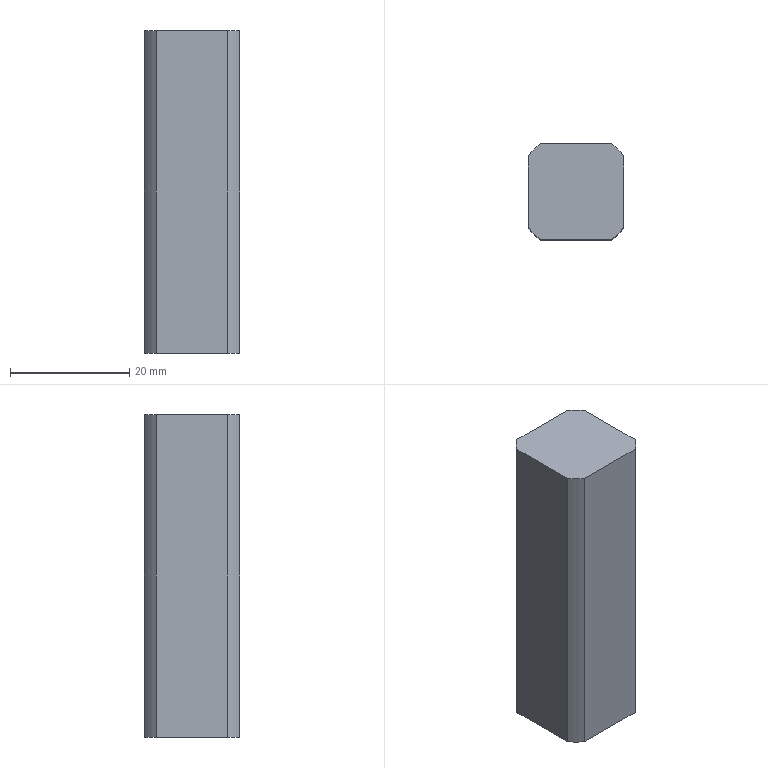Part | STEP file | _CKZT40_ARM.stp | 1 solid | 10 faces | box 16 x 16 x 54 mm | volume 13433 mm3 | plane 6 | cylinder 4 | commonest cylinder face diameters 20 x4
STEP:
#1=CARTESIAN_POINT('',(0.,0.,0.));
#2=DIRECTION('',(0.,0.,1.));
#3=DIRECTION('',(1.,0.,0.));
#4=AXIS2_PLACEMENT_3D('',#1,#2,#3);
#5=CARTESIAN_POINT('',(-6.,8.,27.));
#6=VERTEX_POINT('',#5);
#7=CARTESIAN_POINT('',(-8.,6.,27.));
#8=VERTEX_POINT('',#7);
#9=CARTESIAN_POINT('',(0.,0.,27.));
#10=DIRECTION('',(0.,0.,1.));
#11=DIRECTION('',(1.,0.,0.));
#12=AXIS2_PLACEMENT_3D('',#9,#10,#11);
#13=CIRCLE('',#12,10.);
#14=CARTESIAN_POINT('',(-8.8,-8.8,27.));
#15=DIRECTION('',(0.,0.,1.));
#16=DIRECTION('',(1.,0.,0.));
#17=AXIS2_PLACEMENT_3D('',#14,#15,#16);
#18=PLANE('',#17);
#19=CARTESIAN_POINT('',(8.8,8.8));
#20=DIRECTION('',(1.,0.));
#21=AXIS2_PLACEMENT_2D('',#19,#20);
#22=CIRCLE('',#21,10.);
#23=(GEOMETRIC_REPRESENTATION_CONTEXT(2)PARAMETRIC_REPRESENTATION_CONTEXT()REPRESENTATION_CONTEXT('',''));
#24=DEFINITIONAL_REPRESENTATION('',(#22),#23);
#25=PCURVE('',#18,#24);
#26=CARTESIAN_POINT('',(0.,0.,-29.7));
#27=DIRECTION('',(0.,0.,1.));
#28=DIRECTION('',(-1.,0.,0.));
#29=AXIS2_PLACEMENT_3D('',#26,#27,#28);
#30=CYLINDRICAL_SURFACE('',#29,10.);
#31=CARTESIAN_POINT('',(3.142,56.7));
#32=DIRECTION('',(1.,0.));
#33=VECTOR('',#32,1.);
#34=LINE('',#31,#33);
#35=(GEOMETRIC_REPRESENTATION_CONTEXT(2)PARAMETRIC_REPRESENTATION_CONTEXT()REPRESENTATION_CONTEXT('',''));
#36=DEFINITIONAL_REPRESENTATION('',(#34),#35);
#37=PCURVE('',#30,#36);
#38=SURFACE_CURVE('',#13,(#25,#37),.PCURVE_S1.);
#39=EDGE_CURVE('',#6,#8,#38,.T.);
#40=ORIENTED_EDGE('',*,*,#39,.T.);
#41=CARTESIAN_POINT('',(-8.,-6.,27.));
#42=VERTEX_POINT('',#41);
#43=CARTESIAN_POINT('',(-8.,6.,27.));
#44=DIRECTION('',(0.,-1.,0.));
#45=VECTOR('',#44,1.);
#46=LINE('',#43,#45);
#47=CARTESIAN_POINT('',(0.8,14.8));
#48=DIRECTION('',(0.,-1.));
#49=VECTOR('',#48,1.);
#50=LINE('',#47,#49);
#51=(GEOMETRIC_REPRESENTATION_CONTEXT(2)PARAMETRIC_REPRESENTATION_CONTEXT()REPRESENTATION_CONTEXT('',''));
#52=DEFINITIONAL_REPRESENTATION('',(#50),#51);
#53=PCURVE('',#18,#52);
#54=CARTESIAN_POINT('',(-8.,-6.6,29.7));
#55=DIRECTION('',(1.,0.,0.));
#56=DIRECTION('',(0.,1.,0.));
#57=AXIS2_PLACEMENT_3D('',#54,#55,#56);
#58=PLANE('',#57);
#59=CARTESIAN_POINT('',(12.6,-2.7));
#60=DIRECTION('',(-1.,0.));
#61=VECTOR('',#60,1.);
#62=LINE('',#59,#61);
#63=(GEOMETRIC_REPRESENTATION_CONTEXT(2)PARAMETRIC_REPRESENTATION_CONTEXT()REPRESENTATION_CONTEXT('',''));
#64=DEFINITIONAL_REPRESENTATION('',(#62),#63);
#65=PCURVE('',#58,#64);
#66=SURFACE_CURVE('',#46,(#53,#65),.PCURVE_S1.);
#67=EDGE_CURVE('',#8,#42,#66,.T.);
#68=ORIENTED_EDGE('',*,*,#67,.T.);
#69=CARTESIAN_POINT('',(-6.,-8.,27.));
#70=VERTEX_POINT('',#69);
#71=CARTESIAN_POINT('',(0.,0.,27.));
#72=DIRECTION('',(0.,0.,1.));
#73=DIRECTION('',(1.,0.,0.));
#74=AXIS2_PLACEMENT_3D('',#71,#72,#73);
#75=CIRCLE('',#74,10.);
#76=CARTESIAN_POINT('',(8.8,8.8));
#77=DIRECTION('',(1.,0.));
#78=AXIS2_PLACEMENT_2D('',#76,#77);
#79=CIRCLE('',#78,10.);
#80=(GEOMETRIC_REPRESENTATION_CONTEXT(2)PARAMETRIC_REPRESENTATION_CONTEXT()REPRESENTATION_CONTEXT('',''));
#81=DEFINITIONAL_REPRESENTATION('',(#79),#80);
#82=PCURVE('',#18,#81);
#83=CARTESIAN_POINT('',(0.,0.,-29.7));
#84=DIRECTION('',(0.,0.,1.));
#85=DIRECTION('',(-1.,0.,0.));
#86=AXIS2_PLACEMENT_3D('',#83,#84,#85);
#87=CYLINDRICAL_SURFACE('',#86,10.);
#88=CARTESIAN_POINT('',(-3.142,56.7));
#89=DIRECTION('',(1.,0.));
#90=VECTOR('',#89,1.);
#91=LINE('',#88,#90);
#92=(GEOMETRIC_REPRESENTATION_CONTEXT(2)PARAMETRIC_REPRESENTATION_CONTEXT()REPRESENTATION_CONTEXT('',''));
#93=DEFINITIONAL_REPRESENTATION('',(#91),#92);
#94=PCURVE('',#87,#93);
#95=SURFACE_CURVE('',#75,(#82,#94),.PCURVE_S1.);
#96=EDGE_CURVE('',#42,#70,#95,.T.);
#97=ORIENTED_EDGE('',*,*,#96,.T.);
#98=CARTESIAN_POINT('',(6.,-8.,27.));
#99=VERTEX_POINT('',#98);
#100=CARTESIAN_POINT('',(-6.,-8.,27.));
#101=DIRECTION('',(1.,0.,0.));
#102=VECTOR('',#101,1.);
#103=LINE('',#100,#102);
#104=CARTESIAN_POINT('',(2.8,0.8));
#105=DIRECTION('',(1.,0.));
#106=VECTOR('',#105,1.);
#107=LINE('',#104,#106);
#108=(GEOMETRIC_REPRESENTATION_CONTEXT(2)PARAMETRIC_REPRESENTATION_CONTEXT()REPRESENTATION_CONTEXT('',''));
#109=DEFINITIONAL_REPRESENTATION('',(#107),#108);
#110=PCURVE('',#18,#109);
#111=CARTESIAN_POINT('',(-6.6,-8.,-29.7));
#112=DIRECTION('',(0.,1.,0.));
#113=DIRECTION('',(1.,0.,0.));
#114=AXIS2_PLACEMENT_3D('',#111,#112,#113);
#115=PLANE('',#114);
#116=CARTESIAN_POINT('',(0.6,-56.7));
#117=DIRECTION('',(1.,0.));
#118=VECTOR('',#117,1.);
#119=LINE('',#116,#118);
#120=(GEOMETRIC_REPRESENTATION_CONTEXT(2)PARAMETRIC_REPRESENTATION_CONTEXT()REPRESENTATION_CONTEXT('',''));
#121=DEFINITIONAL_REPRESENTATION('',(#119),#120);
#122=PCURVE('',#115,#121);
#123=SURFACE_CURVE('',#103,(#110,#122),.PCURVE_S1.);
#124=EDGE_CURVE('',#70,#99,#123,.T.);
#125=ORIENTED_EDGE('',*,*,#124,.T.);
#126=CARTESIAN_POINT('',(8.,-6.,27.));
#127=VERTEX_POINT('',#126);
#128=CARTESIAN_POINT('',(0.,0.,27.));
#129=DIRECTION('',(0.,0.,1.));
#130=DIRECTION('',(1.,0.,0.));
#131=AXIS2_PLACEMENT_3D('',#128,#129,#130);
#132=CIRCLE('',#131,10.);
#133=CARTESIAN_POINT('',(8.8,8.8));
#134=DIRECTION('',(1.,0.));
#135=AXIS2_PLACEMENT_2D('',#133,#134);
#136=CIRCLE('',#135,10.);
#137=(GEOMETRIC_REPRESENTATION_CONTEXT(2)PARAMETRIC_REPRESENTATION_CONTEXT()REPRESENTATION_CONTEXT('',''));
#138=DEFINITIONAL_REPRESENTATION('',(#136),#137);
#139=PCURVE('',#18,#138);
#140=CARTESIAN_POINT('',(0.,0.,-29.7));
#141=DIRECTION('',(0.,0.,1.));
#142=DIRECTION('',(-1.,0.,0.));
#143=AXIS2_PLACEMENT_3D('',#140,#141,#142);
#144=CYLINDRICAL_SURFACE('',#143,10.);
#145=CARTESIAN_POINT('',(-3.142,56.7));
#146=DIRECTION('',(1.,0.));
#147=VECTOR('',#146,1.);
#148=LINE('',#145,#147);
#149=(GEOMETRIC_REPRESENTATION_CONTEXT(2)PARAMETRIC_REPRESENTATION_CONTEXT()REPRESENTATION_CONTEXT('',''));
#150=DEFINITIONAL_REPRESENTATION('',(#148),#149);
#151=PCURVE('',#144,#150);
#152=SURFACE_CURVE('',#132,(#139,#151),.PCURVE_S1.);
#153=EDGE_CURVE('',#99,#127,#152,.T.);
#154=ORIENTED_EDGE('',*,*,#153,.T.);
#155=CARTESIAN_POINT('',(8.,6.,27.));
#156=VERTEX_POINT('',#155);
#157=CARTESIAN_POINT('',(8.,-6.,27.));
#158=DIRECTION('',(0.,1.,0.));
#159=VECTOR('',#158,1.);
#160=LINE('',#157,#159);
#161=CARTESIAN_POINT('',(16.8,2.8));
#162=DIRECTION('',(0.,1.));
#163=VECTOR('',#162,1.);
#164=LINE('',#161,#163);
#165=(GEOMETRIC_REPRESENTATION_CONTEXT(2)PARAMETRIC_REPRESENTATION_CONTEXT()REPRESENTATION_CONTEXT('',''));
#166=DEFINITIONAL_REPRESENTATION('',(#164),#165);
#167=PCURVE('',#18,#166);
#168=CARTESIAN_POINT('',(8.,-6.6,-29.7));
#169=DIRECTION('',(-1.,0.,0.));
#170=DIRECTION('',(0.,0.,1.));
#171=AXIS2_PLACEMENT_3D('',#168,#169,#170);
#172=PLANE('',#171);
#173=CARTESIAN_POINT('',(56.7,0.6));
#174=DIRECTION('',(0.,1.));
#175=VECTOR('',#174,1.);
#176=LINE('',#173,#175);
#177=(GEOMETRIC_REPRESENTATION_CONTEXT(2)PARAMETRIC_REPRESENTATION_CONTEXT()REPRESENTATION_CONTEXT('',''));
#178=DEFINITIONAL_REPRESENTATION('',(#176),#177);
#179=PCURVE('',#172,#178);
#180=SURFACE_CURVE('',#160,(#167,#179),.PCURVE_S1.);
#181=EDGE_CURVE('',#127,#156,#180,.T.);
#182=ORIENTED_EDGE('',*,*,#181,.T.);
#183=CARTESIAN_POINT('',(6.,8.,27.));
#184=VERTEX_POINT('',#183);
#185=CARTESIAN_POINT('',(0.,0.,27.));
#186=DIRECTION('',(0.,0.,1.));
#187=DIRECTION('',(1.,0.,0.));
#188=AXIS2_PLACEMENT_3D('',#185,#186,#187);
#189=CIRCLE('',#188,10.);
#190=CARTESIAN_POINT('',(8.8,8.8));
#191=DIRECTION('',(1.,0.));
#192=AXIS2_PLACEMENT_2D('',#190,#191);
#193=CIRCLE('',#192,10.);
#194=(GEOMETRIC_REPRESENTATION_CONTEXT(2)PARAMETRIC_REPRESENTATION_CONTEXT()REPRESENTATION_CONTEXT('',''));
#195=DEFINITIONAL_REPRESENTATION('',(#193),#194);
#196=PCURVE('',#18,#195);
#197=CARTESIAN_POINT('',(0.,0.,-29.7));
#198=DIRECTION('',(0.,0.,1.));
#199=DIRECTION('',(-1.,0.,0.));
#200=AXIS2_PLACEMENT_3D('',#197,#198,#199);
#201=CYLINDRICAL_SURFACE('',#200,10.);
#202=CARTESIAN_POINT('',(3.142,56.7));
#203=DIRECTION('',(1.,0.));
#204=VECTOR('',#203,1.);
#205=LINE('',#202,#204);
#206=(GEOMETRIC_REPRESENTATION_CONTEXT(2)PARAMETRIC_REPRESENTATION_CONTEXT()REPRESENTATION_CONTEXT('',''));
#207=DEFINITIONAL_REPRESENTATION('',(#205),#206);
#208=PCURVE('',#201,#207);
#209=SURFACE_CURVE('',#189,(#196,#208),.PCURVE_S1.);
#210=EDGE_CURVE('',#156,#184,#209,.T.);
#211=ORIENTED_EDGE('',*,*,#210,.T.);
#212=CARTESIAN_POINT('',(6.,8.,27.));
#213=DIRECTION('',(-1.,0.,0.));
#214=VECTOR('',#213,1.);
#215=LINE('',#212,#214);
#216=CARTESIAN_POINT('',(14.8,16.8));
#217=DIRECTION('',(-1.,0.));
#218=VECTOR('',#217,1.);
#219=LINE('',#216,#218);
#220=(GEOMETRIC_REPRESENTATION_CONTEXT(2)PARAMETRIC_REPRESENTATION_CONTEXT()REPRESENTATION_CONTEXT('',''));
#221=DEFINITIONAL_REPRESENTATION('',(#219),#220);
#222=PCURVE('',#18,#221);
#223=CARTESIAN_POINT('',(-6.6,8.,29.7));
#224=DIRECTION('',(0.,-1.,0.));
#225=DIRECTION('',(0.,0.,-1.));
#226=AXIS2_PLACEMENT_3D('',#223,#224,#225);
#227=PLANE('',#226);
#228=CARTESIAN_POINT('',(2.7,12.6));
#229=DIRECTION('',(0.,-1.));
#230=VECTOR('',#229,1.);
#231=LINE('',#228,#230);
#232=(GEOMETRIC_REPRESENTATION_CONTEXT(2)PARAMETRIC_REPRESENTATION_CONTEXT()REPRESENTATION_CONTEXT('',''));
#233=DEFINITIONAL_REPRESENTATION('',(#231),#232);
#234=PCURVE('',#227,#233);
#235=SURFACE_CURVE('',#215,(#222,#234),.PCURVE_S1.);
#236=EDGE_CURVE('',#184,#6,#235,.T.);
#237=ORIENTED_EDGE('',*,*,#236,.T.);
#238=EDGE_LOOP('',(#40,#68,#97,#125,#154,#182,#211,#237));
#239=FACE_BOUND('',#238,.T.);
#240=ADVANCED_FACE('',(#239),#18,.T.);
#241=CARTESIAN_POINT('',(-6.,8.,-27.));
#242=VERTEX_POINT('',#241);
#243=CARTESIAN_POINT('',(-8.,6.,-27.));
#244=VERTEX_POINT('',#243);
#245=CARTESIAN_POINT('',(0.,0.,-27.));
#246=DIRECTION('',(0.,0.,1.));
#247=DIRECTION('',(1.,0.,0.));
#248=AXIS2_PLACEMENT_3D('',#245,#246,#247);
#249=CIRCLE('',#248,10.);
#250=CARTESIAN_POINT('',(-8.8,-8.8,-27.));
#251=DIRECTION('',(0.,0.,1.));
#252=DIRECTION('',(1.,0.,0.));
#253=AXIS2_PLACEMENT_3D('',#250,#251,#252);
#254=PLANE('',#253);
#255=CARTESIAN_POINT('',(8.8,8.8));
#256=DIRECTION('',(1.,0.));
#257=AXIS2_PLACEMENT_2D('',#255,#256);
#258=CIRCLE('',#257,10.);
#259=(GEOMETRIC_REPRESENTATION_CONTEXT(2)PARAMETRIC_REPRESENTATION_CONTEXT()REPRESENTATION_CONTEXT('',''));
#260=DEFINITIONAL_REPRESENTATION('',(#258),#259);
#261=PCURVE('',#254,#260);
#262=CARTESIAN_POINT('',(3.142,2.7));
#263=DIRECTION('',(1.,0.));
#264=VECTOR('',#263,1.);
#265=LINE('',#262,#264);
#266=(GEOMETRIC_REPRESENTATION_CONTEXT(2)PARAMETRIC_REPRESENTATION_CONTEXT()REPRESENTATION_CONTEXT('',''));
#267=DEFINITIONAL_REPRESENTATION('',(#265),#266);
#268=PCURVE('',#30,#267);
#269=SURFACE_CURVE('',#249,(#261,#268),.PCURVE_S1.);
#270=EDGE_CURVE('',#242,#244,#269,.T.);
#271=ORIENTED_EDGE('',*,*,#270,.F.);
#272=CARTESIAN_POINT('',(6.,8.,-27.));
#273=VERTEX_POINT('',#272);
#274=CARTESIAN_POINT('',(6.,8.,-27.));
#275=DIRECTION('',(-1.,0.,0.));
#276=VECTOR('',#275,1.);
#277=LINE('',#274,#276);
#278=CARTESIAN_POINT('',(14.8,16.8));
#279=DIRECTION('',(-1.,0.));
#280=VECTOR('',#279,1.);
#281=LINE('',#278,#280);
#282=(GEOMETRIC_REPRESENTATION_CONTEXT(2)PARAMETRIC_REPRESENTATION_CONTEXT()REPRESENTATION_CONTEXT('',''));
#283=DEFINITIONAL_REPRESENTATION('',(#281),#282);
#284=PCURVE('',#254,#283);
#285=CARTESIAN_POINT('',(56.7,12.6));
#286=DIRECTION('',(0.,-1.));
#287=VECTOR('',#286,1.);
#288=LINE('',#285,#287);
#289=(GEOMETRIC_REPRESENTATION_CONTEXT(2)PARAMETRIC_REPRESENTATION_CONTEXT()REPRESENTATION_CONTEXT('',''));
#290=DEFINITIONAL_REPRESENTATION('',(#288),#289);
#291=PCURVE('',#227,#290);
#292=SURFACE_CURVE('',#277,(#284,#291),.PCURVE_S1.);
#293=EDGE_CURVE('',#273,#242,#292,.T.);
#294=ORIENTED_EDGE('',*,*,#293,.F.);
#295=CARTESIAN_POINT('',(8.,6.,-27.));
#296=VERTEX_POINT('',#295);
#297=CARTESIAN_POINT('',(0.,0.,-27.));
#298=DIRECTION('',(0.,0.,1.));
#299=DIRECTION('',(1.,0.,0.));
#300=AXIS2_PLACEMENT_3D('',#297,#298,#299);
#301=CIRCLE('',#300,10.);
#302=CARTESIAN_POINT('',(8.8,8.8));
#303=DIRECTION('',(1.,0.));
#304=AXIS2_PLACEMENT_2D('',#302,#303);
#305=CIRCLE('',#304,10.);
#306=(GEOMETRIC_REPRESENTATION_CONTEXT(2)PARAMETRIC_REPRESENTATION_CONTEXT()REPRESENTATION_CONTEXT('',''));
#307=DEFINITIONAL_REPRESENTATION('',(#305),#306);
#308=PCURVE('',#254,#307);
#309=CARTESIAN_POINT('',(3.142,2.7));
#310=DIRECTION('',(1.,0.));
#311=VECTOR('',#310,1.);
#312=LINE('',#309,#311);
#313=(GEOMETRIC_REPRESENTATION_CONTEXT(2)PARAMETRIC_REPRESENTATION_CONTEXT()REPRESENTATION_CONTEXT('',''));
#314=DEFINITIONAL_REPRESENTATION('',(#312),#313);
#315=PCURVE('',#201,#314);
#316=SURFACE_CURVE('',#301,(#308,#315),.PCURVE_S1.);
#317=EDGE_CURVE('',#296,#273,#316,.T.);
#318=ORIENTED_EDGE('',*,*,#317,.F.);
#319=CARTESIAN_POINT('',(8.,-6.,-27.));
#320=VERTEX_POINT('',#319);
#321=CARTESIAN_POINT('',(8.,-6.,-27.));
#322=DIRECTION('',(0.,1.,0.));
#323=VECTOR('',#322,1.);
#324=LINE('',#321,#323);
#325=CARTESIAN_POINT('',(16.8,2.8));
#326=DIRECTION('',(0.,1.));
#327=VECTOR('',#326,1.);
#328=LINE('',#325,#327);
#329=(GEOMETRIC_REPRESENTATION_CONTEXT(2)PARAMETRIC_REPRESENTATION_CONTEXT()REPRESENTATION_CONTEXT('',''));
#330=DEFINITIONAL_REPRESENTATION('',(#328),#329);
#331=PCURVE('',#254,#330);
#332=CARTESIAN_POINT('',(2.7,0.6));
#333=DIRECTION('',(0.,1.));
#334=VECTOR('',#333,1.);
#335=LINE('',#332,#334);
#336=(GEOMETRIC_REPRESENTATION_CONTEXT(2)PARAMETRIC_REPRESENTATION_CONTEXT()REPRESENTATION_CONTEXT('',''));
#337=DEFINITIONAL_REPRESENTATION('',(#335),#336);
#338=PCURVE('',#172,#337);
#339=SURFACE_CURVE('',#324,(#331,#338),.PCURVE_S1.);
#340=EDGE_CURVE('',#320,#296,#339,.T.);
#341=ORIENTED_EDGE('',*,*,#340,.F.);
#342=CARTESIAN_POINT('',(6.,-8.,-27.));
#343=VERTEX_POINT('',#342);
#344=CARTESIAN_POINT('',(0.,0.,-27.));
#345=DIRECTION('',(0.,0.,1.));
#346=DIRECTION('',(1.,0.,0.));
#347=AXIS2_PLACEMENT_3D('',#344,#345,#346);
#348=CIRCLE('',#347,10.);
#349=CARTESIAN_POINT('',(8.8,8.8));
#350=DIRECTION('',(1.,0.));
#351=AXIS2_PLACEMENT_2D('',#349,#350);
#352=CIRCLE('',#351,10.);
#353=(GEOMETRIC_REPRESENTATION_CONTEXT(2)PARAMETRIC_REPRESENTATION_CONTEXT()REPRESENTATION_CONTEXT('',''));
#354=DEFINITIONAL_REPRESENTATION('',(#352),#353);
#355=PCURVE('',#254,#354);
#356=CARTESIAN_POINT('',(-3.142,2.7));
#357=DIRECTION('',(1.,0.));
#358=VECTOR('',#357,1.);
#359=LINE('',#356,#358);
#360=(GEOMETRIC_REPRESENTATION_CONTEXT(2)PARAMETRIC_REPRESENTATION_CONTEXT()REPRESENTATION_CONTEXT('',''));
#361=DEFINITIONAL_REPRESENTATION('',(#359),#360);
#362=PCURVE('',#144,#361);
#363=SURFACE_CURVE('',#348,(#355,#362),.PCURVE_S1.);
#364=EDGE_CURVE('',#343,#320,#363,.T.);
#365=ORIENTED_EDGE('',*,*,#364,.F.);
#366=CARTESIAN_POINT('',(-6.,-8.,-27.));
#367=VERTEX_POINT('',#366);
#368=CARTESIAN_POINT('',(-6.,-8.,-27.));
#369=DIRECTION('',(1.,0.,0.));
#370=VECTOR('',#369,1.);
#371=LINE('',#368,#370);
#372=CARTESIAN_POINT('',(2.8,0.8));
#373=DIRECTION('',(1.,0.));
#374=VECTOR('',#373,1.);
#375=LINE('',#372,#374);
#376=(GEOMETRIC_REPRESENTATION_CONTEXT(2)PARAMETRIC_REPRESENTATION_CONTEXT()REPRESENTATION_CONTEXT('',''));
#377=DEFINITIONAL_REPRESENTATION('',(#375),#376);
#378=PCURVE('',#254,#377);
#379=CARTESIAN_POINT('',(0.6,-2.7));
#380=DIRECTION('',(1.,0.));
#381=VECTOR('',#380,1.);
#382=LINE('',#379,#381);
#383=(GEOMETRIC_REPRESENTATION_CONTEXT(2)PARAMETRIC_REPRESENTATION_CONTEXT()REPRESENTATION_CONTEXT('',''));
#384=DEFINITIONAL_REPRESENTATION('',(#382),#383);
#385=PCURVE('',#115,#384);
#386=SURFACE_CURVE('',#371,(#378,#385),.PCURVE_S1.);
#387=EDGE_CURVE('',#367,#343,#386,.T.);
#388=ORIENTED_EDGE('',*,*,#387,.F.);
#389=CARTESIAN_POINT('',(-8.,-6.,-27.));
#390=VERTEX_POINT('',#389);
#391=CARTESIAN_POINT('',(0.,0.,-27.));
#392=DIRECTION('',(0.,0.,1.));
#393=DIRECTION('',(1.,0.,0.));
#394=AXIS2_PLACEMENT_3D('',#391,#392,#393);
#395=CIRCLE('',#394,10.);
#396=CARTESIAN_POINT('',(8.8,8.8));
#397=DIRECTION('',(1.,0.));
#398=AXIS2_PLACEMENT_2D('',#396,#397);
#399=CIRCLE('',#398,10.);
#400=(GEOMETRIC_REPRESENTATION_CONTEXT(2)PARAMETRIC_REPRESENTATION_CONTEXT()REPRESENTATION_CONTEXT('',''));
#401=DEFINITIONAL_REPRESENTATION('',(#399),#400);
#402=PCURVE('',#254,#401);
#403=CARTESIAN_POINT('',(-3.142,2.7));
#404=DIRECTION('',(1.,0.));
#405=VECTOR('',#404,1.);
#406=LINE('',#403,#405);
#407=(GEOMETRIC_REPRESENTATION_CONTEXT(2)PARAMETRIC_REPRESENTATION_CONTEXT()REPRESENTATION_CONTEXT('',''));
#408=DEFINITIONAL_REPRESENTATION('',(#406),#407);
#409=PCURVE('',#87,#408);
#410=SURFACE_CURVE('',#395,(#402,#409),.PCURVE_S1.);
#411=EDGE_CURVE('',#390,#367,#410,.T.);
#412=ORIENTED_EDGE('',*,*,#411,.F.);
#413=CARTESIAN_POINT('',(-8.,6.,-27.));
#414=DIRECTION('',(0.,-1.,0.));
#415=VECTOR('',#414,1.);
#416=LINE('',#413,#415);
#417=CARTESIAN_POINT('',(0.8,14.8));
#418=DIRECTION('',(0.,-1.));
#419=VECTOR('',#418,1.);
#420=LINE('',#417,#419);
#421=(GEOMETRIC_REPRESENTATION_CONTEXT(2)PARAMETRIC_REPRESENTATION_CONTEXT()REPRESENTATION_CONTEXT('',''));
#422=DEFINITIONAL_REPRESENTATION('',(#420),#421);
#423=PCURVE('',#254,#422);
#424=CARTESIAN_POINT('',(12.6,-56.7));
#425=DIRECTION('',(-1.,0.));
#426=VECTOR('',#425,1.);
#427=LINE('',#424,#426);
#428=(GEOMETRIC_REPRESENTATION_CONTEXT(2)PARAMETRIC_REPRESENTATION_CONTEXT()REPRESENTATION_CONTEXT('',''));
#429=DEFINITIONAL_REPRESENTATION('',(#427),#428);
#430=PCURVE('',#58,#429);
#431=SURFACE_CURVE('',#416,(#423,#430),.PCURVE_S1.);
#432=EDGE_CURVE('',#244,#390,#431,.T.);
#433=ORIENTED_EDGE('',*,*,#432,.F.);
#434=EDGE_LOOP('',(#271,#294,#318,#341,#365,#388,#412,#433));
#435=FACE_BOUND('',#434,.T.);
#436=ADVANCED_FACE('',(#435),#254,.F.);
#437=ORIENTED_EDGE('',*,*,#293,.T.);
#438=CARTESIAN_POINT('',(-6.,8.,27.));
#439=DIRECTION('',(0.,0.,-1.));
#440=VECTOR('',#439,1.);
#441=LINE('',#438,#440);
#442=CARTESIAN_POINT('',(2.7,0.6));
#443=DIRECTION('',(1.,0.));
#444=VECTOR('',#443,1.);
#445=LINE('',#442,#444);
#446=(GEOMETRIC_REPRESENTATION_CONTEXT(2)PARAMETRIC_REPRESENTATION_CONTEXT()REPRESENTATION_CONTEXT('',''));
#447=DEFINITIONAL_REPRESENTATION('',(#445),#446);
#448=PCURVE('',#227,#447);
#449=CARTESIAN_POINT('',(5.356,56.7));
#450=DIRECTION('',(0.,-1.));
#451=VECTOR('',#450,1.);
#452=LINE('',#449,#451);
#453=(GEOMETRIC_REPRESENTATION_CONTEXT(2)PARAMETRIC_REPRESENTATION_CONTEXT()REPRESENTATION_CONTEXT('',''));
#454=DEFINITIONAL_REPRESENTATION('',(#452),#453);
#455=PCURVE('',#30,#454);
#456=SURFACE_CURVE('',#441,(#448,#455),.PCURVE_S1.);
#457=EDGE_CURVE('',#6,#242,#456,.T.);
#458=ORIENTED_EDGE('',*,*,#457,.F.);
#459=ORIENTED_EDGE('',*,*,#236,.F.);
#460=CARTESIAN_POINT('',(6.,8.,27.));
#461=DIRECTION('',(0.,0.,-1.));
#462=VECTOR('',#461,1.);
#463=LINE('',#460,#462);
#464=CARTESIAN_POINT('',(2.7,12.6));
#465=DIRECTION('',(1.,0.));
#466=VECTOR('',#465,1.);
#467=LINE('',#464,#466);
#468=(GEOMETRIC_REPRESENTATION_CONTEXT(2)PARAMETRIC_REPRESENTATION_CONTEXT()REPRESENTATION_CONTEXT('',''));
#469=DEFINITIONAL_REPRESENTATION('',(#467),#468);
#470=PCURVE('',#227,#469);
#471=CARTESIAN_POINT('',(4.069,56.7));
#472=DIRECTION('',(0.,-1.));
#473=VECTOR('',#472,1.);
#474=LINE('',#471,#473);
#475=(GEOMETRIC_REPRESENTATION_CONTEXT(2)PARAMETRIC_REPRESENTATION_CONTEXT()REPRESENTATION_CONTEXT('',''));
#476=DEFINITIONAL_REPRESENTATION('',(#474),#475);
#477=PCURVE('',#201,#476);
#478=SURFACE_CURVE('',#463,(#470,#477),.PCURVE_S1.);
#479=EDGE_CURVE('',#184,#273,#478,.T.);
#480=ORIENTED_EDGE('',*,*,#479,.T.);
#481=EDGE_LOOP('',(#437,#458,#459,#480));
#482=FACE_BOUND('',#481,.T.);
#483=ADVANCED_FACE('',(#482),#227,.F.);
#484=ORIENTED_EDGE('',*,*,#317,.T.);
#485=ORIENTED_EDGE('',*,*,#479,.F.);
#486=ORIENTED_EDGE('',*,*,#210,.F.);
#487=CARTESIAN_POINT('',(8.,6.,27.));
#488=DIRECTION('',(0.,0.,-1.));
#489=VECTOR('',#488,1.);
#490=LINE('',#487,#489);
#491=CARTESIAN_POINT('',(3.785,56.7));
#492=DIRECTION('',(0.,-1.));
#493=VECTOR('',#492,1.);
#494=LINE('',#491,#493);
#495=(GEOMETRIC_REPRESENTATION_CONTEXT(2)PARAMETRIC_REPRESENTATION_CONTEXT()REPRESENTATION_CONTEXT('',''));
#496=DEFINITIONAL_REPRESENTATION('',(#494),#495);
#497=PCURVE('',#201,#496);
#498=CARTESIAN_POINT('',(56.7,12.6));
#499=DIRECTION('',(-1.,0.));
#500=VECTOR('',#499,1.);
#501=LINE('',#498,#500);
#502=(GEOMETRIC_REPRESENTATION_CONTEXT(2)PARAMETRIC_REPRESENTATION_CONTEXT()REPRESENTATION_CONTEXT('',''));
#503=DEFINITIONAL_REPRESENTATION('',(#501),#502);
#504=PCURVE('',#172,#503);
#505=SURFACE_CURVE('',#490,(#497,#504),.PCURVE_S1.);
#506=EDGE_CURVE('',#156,#296,#505,.T.);
#507=ORIENTED_EDGE('',*,*,#506,.T.);
#508=EDGE_LOOP('',(#484,#485,#486,#507));
#509=FACE_BOUND('',#508,.T.);
#510=ADVANCED_FACE('',(#509),#201,.T.);
#511=ORIENTED_EDGE('',*,*,#340,.T.);
#512=ORIENTED_EDGE('',*,*,#506,.F.);
#513=ORIENTED_EDGE('',*,*,#181,.F.);
#514=CARTESIAN_POINT('',(8.,-6.,27.));
#515=DIRECTION('',(0.,0.,-1.));
#516=VECTOR('',#515,1.);
#517=LINE('',#514,#516);
#518=CARTESIAN_POINT('',(56.7,0.6));
#519=DIRECTION('',(-1.,0.));
#520=VECTOR('',#519,1.);
#521=LINE('',#518,#520);
#522=(GEOMETRIC_REPRESENTATION_CONTEXT(2)PARAMETRIC_REPRESENTATION_CONTEXT()REPRESENTATION_CONTEXT('',''));
#523=DEFINITIONAL_REPRESENTATION('',(#521),#522);
#524=PCURVE('',#172,#523);
#525=CARTESIAN_POINT('',(2.498,56.7));
#526=DIRECTION('',(0.,-1.));
#527=VECTOR('',#526,1.);
#528=LINE('',#525,#527);
#529=(GEOMETRIC_REPRESENTATION_CONTEXT(2)PARAMETRIC_REPRESENTATION_CONTEXT()REPRESENTATION_CONTEXT('',''));
#530=DEFINITIONAL_REPRESENTATION('',(#528),#529);
#531=PCURVE('',#144,#530);
#532=SURFACE_CURVE('',#517,(#524,#531),.PCURVE_S1.);
#533=EDGE_CURVE('',#127,#320,#532,.T.);
#534=ORIENTED_EDGE('',*,*,#533,.T.);
#535=EDGE_LOOP('',(#511,#512,#513,#534));
#536=FACE_BOUND('',#535,.T.);
#537=ADVANCED_FACE('',(#536),#172,.F.);
#538=ORIENTED_EDGE('',*,*,#364,.T.);
#539=ORIENTED_EDGE('',*,*,#533,.F.);
#540=ORIENTED_EDGE('',*,*,#153,.F.);
#541=CARTESIAN_POINT('',(6.,-8.,27.));
#542=DIRECTION('',(0.,0.,-1.));
#543=VECTOR('',#542,1.);
#544=LINE('',#541,#543);
#545=CARTESIAN_POINT('',(2.214,56.7));
#546=DIRECTION('',(0.,-1.));
#547=VECTOR('',#546,1.);
#548=LINE('',#545,#547);
#549=(GEOMETRIC_REPRESENTATION_CONTEXT(2)PARAMETRIC_REPRESENTATION_CONTEXT()REPRESENTATION_CONTEXT('',''));
#550=DEFINITIONAL_REPRESENTATION('',(#548),#549);
#551=PCURVE('',#144,#550);
#552=CARTESIAN_POINT('',(12.6,-56.7));
#553=DIRECTION('',(0.,1.));
#554=VECTOR('',#553,1.);
#555=LINE('',#552,#554);
#556=(GEOMETRIC_REPRESENTATION_CONTEXT(2)PARAMETRIC_REPRESENTATION_CONTEXT()REPRESENTATION_CONTEXT('',''));
#557=DEFINITIONAL_REPRESENTATION('',(#555),#556);
#558=PCURVE('',#115,#557);
#559=SURFACE_CURVE('',#544,(#551,#558),.PCURVE_S1.);
#560=EDGE_CURVE('',#99,#343,#559,.T.);
#561=ORIENTED_EDGE('',*,*,#560,.T.);
#562=EDGE_LOOP('',(#538,#539,#540,#561));
#563=FACE_BOUND('',#562,.T.);
#564=ADVANCED_FACE('',(#563),#144,.T.);
#565=ORIENTED_EDGE('',*,*,#387,.T.);
#566=ORIENTED_EDGE('',*,*,#560,.F.);
#567=ORIENTED_EDGE('',*,*,#124,.F.);
#568=CARTESIAN_POINT('',(-6.,-8.,27.));
#569=DIRECTION('',(0.,0.,-1.));
#570=VECTOR('',#569,1.);
#571=LINE('',#568,#570);
#572=CARTESIAN_POINT('',(0.6,-56.7));
#573=DIRECTION('',(0.,1.));
#574=VECTOR('',#573,1.);
#575=LINE('',#572,#574);
#576=(GEOMETRIC_REPRESENTATION_CONTEXT(2)PARAMETRIC_REPRESENTATION_CONTEXT()REPRESENTATION_CONTEXT('',''));
#577=DEFINITIONAL_REPRESENTATION('',(#575),#576);
#578=PCURVE('',#115,#577);
#579=CARTESIAN_POINT('',(0.9273,56.7));
#580=DIRECTION('',(0.,-1.));
#581=VECTOR('',#580,1.);
#582=LINE('',#579,#581);
#583=(GEOMETRIC_REPRESENTATION_CONTEXT(2)PARAMETRIC_REPRESENTATION_CONTEXT()REPRESENTATION_CONTEXT('',''));
#584=DEFINITIONAL_REPRESENTATION('',(#582),#583);
#585=PCURVE('',#87,#584);
#586=SURFACE_CURVE('',#571,(#578,#585),.PCURVE_S1.);
#587=EDGE_CURVE('',#70,#367,#586,.T.);
#588=ORIENTED_EDGE('',*,*,#587,.T.);
#589=EDGE_LOOP('',(#565,#566,#567,#588));
#590=FACE_BOUND('',#589,.T.);
#591=ADVANCED_FACE('',(#590),#115,.F.);
#592=ORIENTED_EDGE('',*,*,#270,.T.);
#593=CARTESIAN_POINT('',(-8.,6.,27.));
#594=DIRECTION('',(0.,0.,-1.));
#595=VECTOR('',#594,1.);
#596=LINE('',#593,#595);
#597=CARTESIAN_POINT('',(5.64,56.7));
#598=DIRECTION('',(0.,-1.));
#599=VECTOR('',#598,1.);
#600=LINE('',#597,#599);
#601=(GEOMETRIC_REPRESENTATION_CONTEXT(2)PARAMETRIC_REPRESENTATION_CONTEXT()REPRESENTATION_CONTEXT('',''));
#602=DEFINITIONAL_REPRESENTATION('',(#600),#601);
#603=PCURVE('',#30,#602);
#604=CARTESIAN_POINT('',(12.6,-2.7));
#605=DIRECTION('',(0.,-1.));
#606=VECTOR('',#605,1.);
#607=LINE('',#604,#606);
#608=(GEOMETRIC_REPRESENTATION_CONTEXT(2)PARAMETRIC_REPRESENTATION_CONTEXT()REPRESENTATION_CONTEXT('',''));
#609=DEFINITIONAL_REPRESENTATION('',(#607),#608);
#610=PCURVE('',#58,#609);
#611=SURFACE_CURVE('',#596,(#603,#610),.PCURVE_S1.);
#612=EDGE_CURVE('',#8,#244,#611,.T.);
#613=ORIENTED_EDGE('',*,*,#612,.F.);
#614=ORIENTED_EDGE('',*,*,#39,.F.);
#615=ORIENTED_EDGE('',*,*,#457,.T.);
#616=EDGE_LOOP('',(#592,#613,#614,#615));
#617=FACE_BOUND('',#616,.T.);
#618=ADVANCED_FACE('',(#617),#30,.T.);
#619=ORIENTED_EDGE('',*,*,#411,.T.);
#620=ORIENTED_EDGE('',*,*,#587,.F.);
#621=ORIENTED_EDGE('',*,*,#96,.F.);
#622=CARTESIAN_POINT('',(-8.,-6.,27.));
#623=DIRECTION('',(0.,0.,-1.));
#624=VECTOR('',#623,1.);
#625=LINE('',#622,#624);
#626=CARTESIAN_POINT('',(0.6435,56.7));
#627=DIRECTION('',(0.,-1.));
#628=VECTOR('',#627,1.);
#629=LINE('',#626,#628);
#630=(GEOMETRIC_REPRESENTATION_CONTEXT(2)PARAMETRIC_REPRESENTATION_CONTEXT()REPRESENTATION_CONTEXT('',''));
#631=DEFINITIONAL_REPRESENTATION('',(#629),#630);
#632=PCURVE('',#87,#631);
#633=CARTESIAN_POINT('',(0.6,-2.7));
#634=DIRECTION('',(0.,-1.));
#635=VECTOR('',#634,1.);
#636=LINE('',#633,#635);
#637=(GEOMETRIC_REPRESENTATION_CONTEXT(2)PARAMETRIC_REPRESENTATION_CONTEXT()REPRESENTATION_CONTEXT('',''));
#638=DEFINITIONAL_REPRESENTATION('',(#636),#637);
#639=PCURVE('',#58,#638);
#640=SURFACE_CURVE('',#625,(#632,#639),.PCURVE_S1.);
#641=EDGE_CURVE('',#42,#390,#640,.T.);
#642=ORIENTED_EDGE('',*,*,#641,.T.);
#643=EDGE_LOOP('',(#619,#620,#621,#642));
#644=FACE_BOUND('',#643,.T.);
#645=ADVANCED_FACE('',(#644),#87,.T.);
#646=ORIENTED_EDGE('',*,*,#432,.T.);
#647=ORIENTED_EDGE('',*,*,#641,.F.);
#648=ORIENTED_EDGE('',*,*,#67,.F.);
#649=ORIENTED_EDGE('',*,*,#612,.T.);
#650=EDGE_LOOP('',(#646,#647,#648,#649));
#651=FACE_BOUND('',#650,.T.);
#652=ADVANCED_FACE('',(#651),#58,.F.);
#653=CLOSED_SHELL('',(#240,#436,#483,#510,#537,#564,#591,#618,#645,#652));
#654=MANIFOLD_SOLID_BREP('',#653);
#655=(LENGTH_UNIT()NAMED_UNIT(*)SI_UNIT(.MILLI.,.METRE.));
#656=UNCERTAINTY_MEASURE_WITH_UNIT(LENGTH_MEASURE(0.0000001),#655,'','');
#657=(NAMED_UNIT(*)PLANE_ANGLE_UNIT()SI_UNIT($,.RADIAN.));
#658=(NAMED_UNIT(*)SI_UNIT($,.STERADIAN.)SOLID_ANGLE_UNIT());
#659=(GEOMETRIC_REPRESENTATION_CONTEXT(3)GLOBAL_UNCERTAINTY_ASSIGNED_CONTEXT((#656))GLOBAL_UNIT_ASSIGNED_CONTEXT((#655,#657,#658))REPRESENTATION_CONTEXT('',''));
#660=ADVANCED_BREP_SHAPE_REPRESENTATION('',(#4,#654),#659);